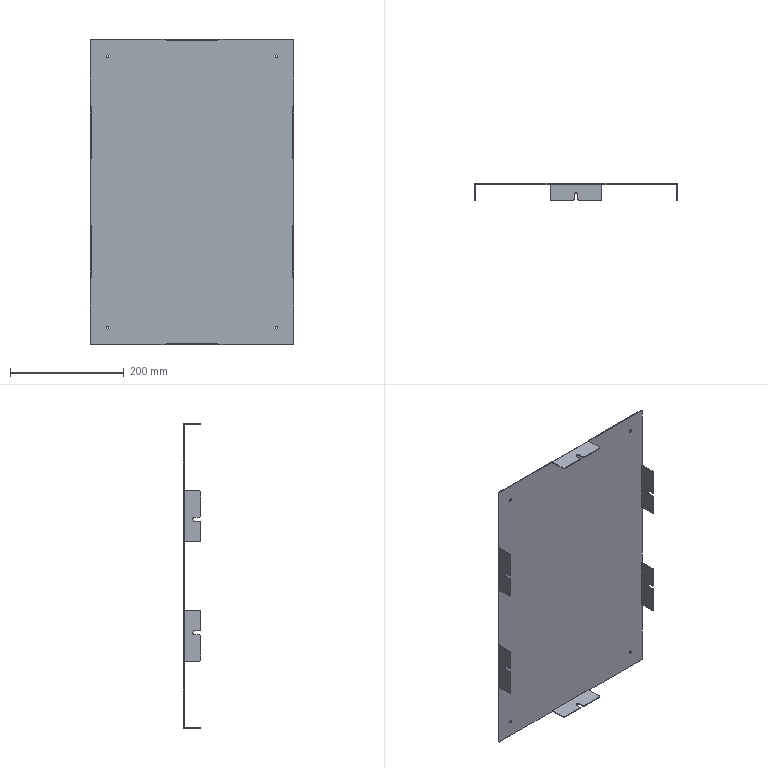Part | STEP file | Cabinet sheet-metal cover plate A | 1 solid | 168 faces | box 358 x 30 x 538 mm | volume 310725 mm3 | plane 108 | cylinder 60 | commonest cylinder face diameters 4 x28 7 x12 5 x8 0.1 x6 3.1 x6